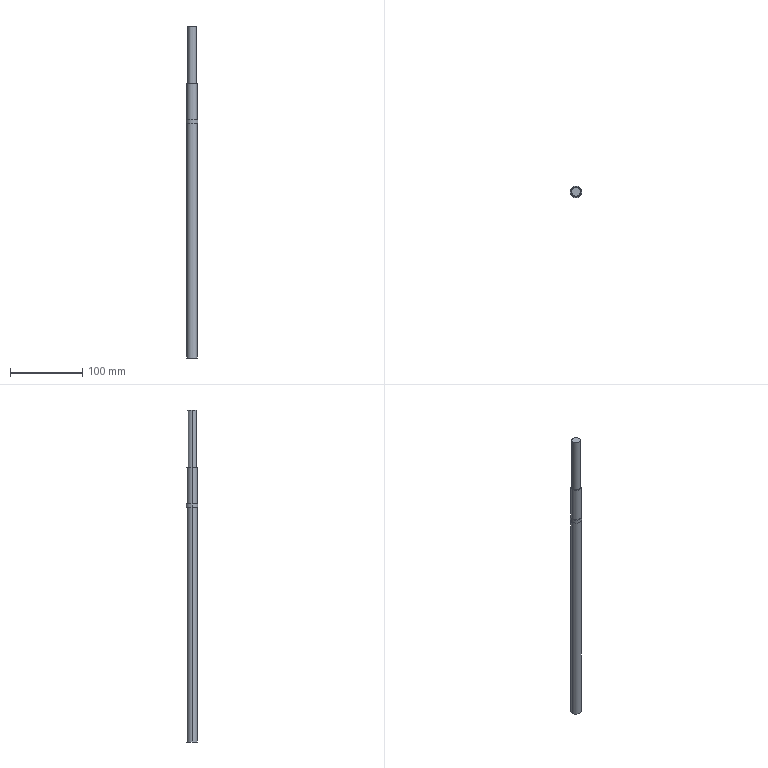Part | SolidWorks | features MirrorStock 1 | 1 solid | 13 faces | box 16 x 16 x 460 mm | volume 67780 mm3 | cylinder 8 | plane 5 | commonest cylinder face diameters 14 x4 12 x2 16 x2
STEP:
#1=CARTESIAN_POINT('',(-7.,0.,-460.));
#2=VERTEX_POINT('',#1);
#3=CARTESIAN_POINT('',(7.,0.,-460.));
#4=VERTEX_POINT('',#3);
#5=CARTESIAN_POINT('',(0.,0.,-460.));
#6=DIRECTION('',(0.,0.,1.));
#7=DIRECTION('',(1.,0.,0.));
#8=AXIS2_PLACEMENT_3D('',#5,#6,#7);
#9=CIRCLE('',#8,7.);
#10=EDGE_CURVE('',#2,#4,#9,.T.);
#11=ORIENTED_EDGE('',*,*,#10,.T.);
#12=CARTESIAN_POINT('',(7.,0.,-135.));
#13=VERTEX_POINT('',#12);
#14=CARTESIAN_POINT('',(7.,0.,-460.));
#15=DIRECTION('',(0.,0.,1.));
#16=VECTOR('',#15,1000.);
#17=LINE('',#14,#16);
#18=EDGE_CURVE('',#4,#13,#17,.T.);
#19=ORIENTED_EDGE('',*,*,#18,.T.);
#20=CARTESIAN_POINT('',(-7.,0.,-135.));
#21=VERTEX_POINT('',#20);
#22=CARTESIAN_POINT('',(0.,0.,-135.));
#23=DIRECTION('',(0.,0.,1.));
#24=DIRECTION('',(1.,0.,0.));
#25=AXIS2_PLACEMENT_3D('',#22,#23,#24);
#26=CIRCLE('',#25,7.);
#27=EDGE_CURVE('',#21,#13,#26,.T.);
#28=ORIENTED_EDGE('',*,*,#27,.F.);
#29=CARTESIAN_POINT('',(-7.,0.,-460.));
#30=DIRECTION('',(0.,0.,1.));
#31=VECTOR('',#30,1000.);
#32=LINE('',#29,#31);
#33=EDGE_CURVE('',#2,#21,#32,.T.);
#34=ORIENTED_EDGE('',*,*,#33,.F.);
#35=EDGE_LOOP('',(#11,#19,#28,#34));
#36=FACE_OUTER_BOUND('',#35,.T.);
#37=CARTESIAN_POINT('',(0.,0.,-460.));
#38=DIRECTION('',(0.,0.,1.));
#39=DIRECTION('',(-1.,0.,0.));
#40=AXIS2_PLACEMENT_3D('',#37,#38,#39);
#41=CYLINDRICAL_SURFACE('',#40,7.);
#42=ADVANCED_FACE('',(#36),#41,.T.);
#43=CARTESIAN_POINT('',(-8.,0.,-135.));
#44=VERTEX_POINT('',#43);
#45=CARTESIAN_POINT('',(8.,0.,-135.));
#46=VERTEX_POINT('',#45);
#47=CARTESIAN_POINT('',(0.,0.,-135.));
#48=DIRECTION('',(0.,0.,1.));
#49=DIRECTION('',(1.,0.,0.));
#50=AXIS2_PLACEMENT_3D('',#47,#48,#49);
#51=CIRCLE('',#50,8.);
#52=EDGE_CURVE('',#44,#46,#51,.T.);
#53=ORIENTED_EDGE('',*,*,#52,.T.);
#54=CARTESIAN_POINT('',(8.,0.,-130.));
#55=VERTEX_POINT('',#54);
#56=CARTESIAN_POINT('',(8.,0.,-135.));
#57=DIRECTION('',(0.,0.,1.));
#58=VECTOR('',#57,1000.);
#59=LINE('',#56,#58);
#60=EDGE_CURVE('',#46,#55,#59,.T.);
#61=ORIENTED_EDGE('',*,*,#60,.T.);
#62=CARTESIAN_POINT('',(-8.,0.,-130.));
#63=VERTEX_POINT('',#62);
#64=CARTESIAN_POINT('',(0.,0.,-130.));
#65=DIRECTION('',(0.,0.,1.));
#66=DIRECTION('',(1.,0.,0.));
#67=AXIS2_PLACEMENT_3D('',#64,#65,#66);
#68=CIRCLE('',#67,8.);
#69=EDGE_CURVE('',#63,#55,#68,.T.);
#70=ORIENTED_EDGE('',*,*,#69,.F.);
#71=CARTESIAN_POINT('',(-8.,0.,-135.));
#72=DIRECTION('',(0.,0.,1.));
#73=VECTOR('',#72,1000.);
#74=LINE('',#71,#73);
#75=EDGE_CURVE('',#44,#63,#74,.T.);
#76=ORIENTED_EDGE('',*,*,#75,.F.);
#77=EDGE_LOOP('',(#53,#61,#70,#76));
#78=FACE_OUTER_BOUND('',#77,.T.);
#79=CARTESIAN_POINT('',(0.,0.,-135.));
#80=DIRECTION('',(0.,0.,1.));
#81=DIRECTION('',(-1.,0.,0.));
#82=AXIS2_PLACEMENT_3D('',#79,#80,#81);
#83=CYLINDRICAL_SURFACE('',#82,8.);
#84=ADVANCED_FACE('',(#78),#83,.T.);
#85=CARTESIAN_POINT('',(-6.,0.,-80.));
#86=VERTEX_POINT('',#85);
#87=CARTESIAN_POINT('',(6.,0.,-80.));
#88=VERTEX_POINT('',#87);
#89=CARTESIAN_POINT('',(0.,0.,-80.));
#90=DIRECTION('',(0.,0.,1.));
#91=DIRECTION('',(1.,0.,0.));
#92=AXIS2_PLACEMENT_3D('',#89,#90,#91);
#93=CIRCLE('',#92,6.);
#94=EDGE_CURVE('',#86,#88,#93,.T.);
#95=ORIENTED_EDGE('',*,*,#94,.T.);
#96=CARTESIAN_POINT('',(6.,0.,0.));
#97=VERTEX_POINT('',#96);
#98=CARTESIAN_POINT('',(6.,0.,-80.));
#99=DIRECTION('',(0.,0.,1.));
#100=VECTOR('',#99,1000.);
#101=LINE('',#98,#100);
#102=EDGE_CURVE('',#88,#97,#101,.T.);
#103=ORIENTED_EDGE('',*,*,#102,.T.);
#104=CARTESIAN_POINT('',(-6.,0.,0.));
#105=VERTEX_POINT('',#104);
#106=CARTESIAN_POINT('',(0.,0.,0.));
#107=DIRECTION('',(0.,0.,1.));
#108=DIRECTION('',(1.,0.,0.));
#109=AXIS2_PLACEMENT_3D('',#106,#107,#108);
#110=CIRCLE('',#109,6.);
#111=EDGE_CURVE('',#105,#97,#110,.T.);
#112=ORIENTED_EDGE('',*,*,#111,.F.);
#113=CARTESIAN_POINT('',(-6.,0.,-80.));
#114=DIRECTION('',(0.,0.,1.));
#115=VECTOR('',#114,1000.);
#116=LINE('',#113,#115);
#117=EDGE_CURVE('',#86,#105,#116,.T.);
#118=ORIENTED_EDGE('',*,*,#117,.F.);
#119=EDGE_LOOP('',(#95,#103,#112,#118));
#120=FACE_OUTER_BOUND('',#119,.T.);
#121=CARTESIAN_POINT('',(0.,0.,-80.));
#122=DIRECTION('',(0.,0.,1.));
#123=DIRECTION('',(-1.,0.,0.));
#124=AXIS2_PLACEMENT_3D('',#121,#122,#123);
#125=CYLINDRICAL_SURFACE('',#124,6.);
#126=ADVANCED_FACE('',(#120),#125,.T.);
#127=CARTESIAN_POINT('',(-7.,0.,-130.));
#128=VERTEX_POINT('',#127);
#129=CARTESIAN_POINT('',(7.,0.,-130.));
#130=VERTEX_POINT('',#129);
#131=CARTESIAN_POINT('',(0.,0.,-130.));
#132=DIRECTION('',(0.,0.,1.));
#133=DIRECTION('',(1.,0.,0.));
#134=AXIS2_PLACEMENT_3D('',#131,#132,#133);
#135=CIRCLE('',#134,7.);
#136=EDGE_CURVE('',#128,#130,#135,.T.);
#137=ORIENTED_EDGE('',*,*,#136,.T.);
#138=CARTESIAN_POINT('',(7.,0.,-80.));
#139=VERTEX_POINT('',#138);
#140=CARTESIAN_POINT('',(7.,0.,-460.));
#141=DIRECTION('',(0.,0.,1.));
#142=VECTOR('',#141,1000.);
#143=LINE('',#140,#142);
#144=EDGE_CURVE('',#130,#139,#143,.T.);
#145=ORIENTED_EDGE('',*,*,#144,.T.);
#146=CARTESIAN_POINT('',(-7.,0.,-80.));
#147=VERTEX_POINT('',#146);
#148=CARTESIAN_POINT('',(0.,0.,-80.));
#149=DIRECTION('',(0.,0.,1.));
#150=DIRECTION('',(1.,0.,0.));
#151=AXIS2_PLACEMENT_3D('',#148,#149,#150);
#152=CIRCLE('',#151,7.);
#153=EDGE_CURVE('',#147,#139,#152,.T.);
#154=ORIENTED_EDGE('',*,*,#153,.F.);
#155=CARTESIAN_POINT('',(-7.,0.,-460.));
#156=DIRECTION('',(0.,0.,1.));
#157=VECTOR('',#156,1000.);
#158=LINE('',#155,#157);
#159=EDGE_CURVE('',#128,#147,#158,.T.);
#160=ORIENTED_EDGE('',*,*,#159,.F.);
#161=EDGE_LOOP('',(#137,#145,#154,#160));
#162=FACE_OUTER_BOUND('',#161,.T.);
#163=CARTESIAN_POINT('',(0.,0.,-460.));
#164=DIRECTION('',(0.,0.,1.));
#165=DIRECTION('',(-1.,0.,0.));
#166=AXIS2_PLACEMENT_3D('',#163,#164,#165);
#167=CYLINDRICAL_SURFACE('',#166,7.);
#168=ADVANCED_FACE('',(#162),#167,.T.);
#169=ORIENTED_EDGE('',*,*,#144,.F.);
#170=CARTESIAN_POINT('',(0.,0.,-130.));
#171=DIRECTION('',(0.,0.,1.));
#172=DIRECTION('',(1.,0.,0.));
#173=AXIS2_PLACEMENT_3D('',#170,#171,#172);
#174=CIRCLE('',#173,7.);
#175=EDGE_CURVE('',#130,#128,#174,.T.);
#176=ORIENTED_EDGE('',*,*,#175,.T.);
#177=ORIENTED_EDGE('',*,*,#159,.T.);
#178=CARTESIAN_POINT('',(0.,0.,-80.));
#179=DIRECTION('',(0.,0.,1.));
#180=DIRECTION('',(1.,0.,0.));
#181=AXIS2_PLACEMENT_3D('',#178,#179,#180);
#182=CIRCLE('',#181,7.);
#183=EDGE_CURVE('',#139,#147,#182,.T.);
#184=ORIENTED_EDGE('',*,*,#183,.F.);
#185=EDGE_LOOP('',(#169,#176,#177,#184));
#186=FACE_OUTER_BOUND('',#185,.T.);
#187=CARTESIAN_POINT('',(0.,0.,-460.));
#188=DIRECTION('',(0.,0.,1.));
#189=DIRECTION('',(-1.,0.,0.));
#190=AXIS2_PLACEMENT_3D('',#187,#188,#189);
#191=CYLINDRICAL_SURFACE('',#190,7.);
#192=ADVANCED_FACE('',(#186),#191,.T.);
#193=ORIENTED_EDGE('',*,*,#102,.F.);
#194=CARTESIAN_POINT('',(0.,0.,-80.));
#195=DIRECTION('',(0.,0.,1.));
#196=DIRECTION('',(1.,0.,0.));
#197=AXIS2_PLACEMENT_3D('',#194,#195,#196);
#198=CIRCLE('',#197,6.);
#199=EDGE_CURVE('',#88,#86,#198,.T.);
#200=ORIENTED_EDGE('',*,*,#199,.T.);
#201=ORIENTED_EDGE('',*,*,#117,.T.);
#202=CARTESIAN_POINT('',(0.,0.,0.));
#203=DIRECTION('',(0.,0.,1.));
#204=DIRECTION('',(1.,0.,0.));
#205=AXIS2_PLACEMENT_3D('',#202,#203,#204);
#206=CIRCLE('',#205,6.);
#207=EDGE_CURVE('',#97,#105,#206,.T.);
#208=ORIENTED_EDGE('',*,*,#207,.F.);
#209=EDGE_LOOP('',(#193,#200,#201,#208));
#210=FACE_OUTER_BOUND('',#209,.T.);
#211=CARTESIAN_POINT('',(0.,0.,-80.));
#212=DIRECTION('',(0.,0.,1.));
#213=DIRECTION('',(-1.,0.,0.));
#214=AXIS2_PLACEMENT_3D('',#211,#212,#213);
#215=CYLINDRICAL_SURFACE('',#214,6.);
#216=ADVANCED_FACE('',(#210),#215,.T.);
#217=ORIENTED_EDGE('',*,*,#111,.T.);
#218=ORIENTED_EDGE('',*,*,#207,.T.);
#219=EDGE_LOOP('',(#217,#218));
#220=FACE_OUTER_BOUND('',#219,.T.);
#221=CARTESIAN_POINT('',(0.,0.,0.));
#222=DIRECTION('',(0.,0.,-1.));
#223=DIRECTION('',(1.,0.,0.));
#224=AXIS2_PLACEMENT_3D('',#221,#222,#223);
#225=PLANE('',#224);
#226=ADVANCED_FACE('',(#220),#225,.F.);
#227=ORIENTED_EDGE('',*,*,#94,.F.);
#228=ORIENTED_EDGE('',*,*,#199,.F.);
#229=EDGE_LOOP('',(#227,#228));
#230=FACE_BOUND('',#229,.T.);
#231=ORIENTED_EDGE('',*,*,#153,.T.);
#232=ORIENTED_EDGE('',*,*,#183,.T.);
#233=EDGE_LOOP('',(#231,#232));
#234=FACE_OUTER_BOUND('',#233,.T.);
#235=CARTESIAN_POINT('',(0.,0.,-80.));
#236=DIRECTION('',(0.,0.,-1.));
#237=DIRECTION('',(1.,0.,0.));
#238=AXIS2_PLACEMENT_3D('',#235,#236,#237);
#239=PLANE('',#238);
#240=ADVANCED_FACE('',(#230,#234),#239,.F.);
#241=ORIENTED_EDGE('',*,*,#60,.F.);
#242=CARTESIAN_POINT('',(0.,0.,-135.));
#243=DIRECTION('',(0.,0.,1.));
#244=DIRECTION('',(1.,0.,0.));
#245=AXIS2_PLACEMENT_3D('',#242,#243,#244);
#246=CIRCLE('',#245,8.);
#247=EDGE_CURVE('',#46,#44,#246,.T.);
#248=ORIENTED_EDGE('',*,*,#247,.T.);
#249=ORIENTED_EDGE('',*,*,#75,.T.);
#250=CARTESIAN_POINT('',(0.,0.,-130.));
#251=DIRECTION('',(0.,0.,1.));
#252=DIRECTION('',(1.,0.,0.));
#253=AXIS2_PLACEMENT_3D('',#250,#251,#252);
#254=CIRCLE('',#253,8.);
#255=EDGE_CURVE('',#55,#63,#254,.T.);
#256=ORIENTED_EDGE('',*,*,#255,.F.);
#257=EDGE_LOOP('',(#241,#248,#249,#256));
#258=FACE_OUTER_BOUND('',#257,.T.);
#259=CARTESIAN_POINT('',(0.,0.,-135.));
#260=DIRECTION('',(0.,0.,1.));
#261=DIRECTION('',(-1.,0.,0.));
#262=AXIS2_PLACEMENT_3D('',#259,#260,#261);
#263=CYLINDRICAL_SURFACE('',#262,8.);
#264=ADVANCED_FACE('',(#258),#263,.T.);
#265=ORIENTED_EDGE('',*,*,#27,.T.);
#266=CARTESIAN_POINT('',(0.,0.,-135.));
#267=DIRECTION('',(0.,0.,1.));
#268=DIRECTION('',(1.,0.,0.));
#269=AXIS2_PLACEMENT_3D('',#266,#267,#268);
#270=CIRCLE('',#269,7.);
#271=EDGE_CURVE('',#13,#21,#270,.T.);
#272=ORIENTED_EDGE('',*,*,#271,.T.);
#273=EDGE_LOOP('',(#265,#272));
#274=FACE_BOUND('',#273,.T.);
#275=ORIENTED_EDGE('',*,*,#52,.F.);
#276=ORIENTED_EDGE('',*,*,#247,.F.);
#277=EDGE_LOOP('',(#275,#276));
#278=FACE_OUTER_BOUND('',#277,.T.);
#279=CARTESIAN_POINT('',(0.,0.,-135.));
#280=DIRECTION('',(0.,0.,-1.));
#281=DIRECTION('',(1.,0.,0.));
#282=AXIS2_PLACEMENT_3D('',#279,#280,#281);
#283=PLANE('',#282);
#284=ADVANCED_FACE('',(#274,#278),#283,.T.);
#285=ORIENTED_EDGE('',*,*,#136,.F.);
#286=ORIENTED_EDGE('',*,*,#175,.F.);
#287=EDGE_LOOP('',(#285,#286));
#288=FACE_BOUND('',#287,.T.);
#289=ORIENTED_EDGE('',*,*,#69,.T.);
#290=ORIENTED_EDGE('',*,*,#255,.T.);
#291=EDGE_LOOP('',(#289,#290));
#292=FACE_OUTER_BOUND('',#291,.T.);
#293=CARTESIAN_POINT('',(0.,0.,-130.));
#294=DIRECTION('',(0.,0.,-1.));
#295=DIRECTION('',(1.,0.,0.));
#296=AXIS2_PLACEMENT_3D('',#293,#294,#295);
#297=PLANE('',#296);
#298=ADVANCED_FACE('',(#288,#292),#297,.F.);
#299=ORIENTED_EDGE('',*,*,#10,.F.);
#300=CARTESIAN_POINT('',(0.,0.,-460.));
#301=DIRECTION('',(0.,0.,1.));
#302=DIRECTION('',(1.,0.,0.));
#303=AXIS2_PLACEMENT_3D('',#300,#301,#302);
#304=CIRCLE('',#303,7.);
#305=EDGE_CURVE('',#4,#2,#304,.T.);
#306=ORIENTED_EDGE('',*,*,#305,.F.);
#307=EDGE_LOOP('',(#299,#306));
#308=FACE_OUTER_BOUND('',#307,.T.);
#309=CARTESIAN_POINT('',(0.,0.,-460.));
#310=DIRECTION('',(0.,0.,-1.));
#311=DIRECTION('',(1.,0.,0.));
#312=AXIS2_PLACEMENT_3D('',#309,#310,#311);
#313=PLANE('',#312);
#314=ADVANCED_FACE('',(#308),#313,.T.);
#315=ORIENTED_EDGE('',*,*,#18,.F.);
#316=ORIENTED_EDGE('',*,*,#305,.T.);
#317=ORIENTED_EDGE('',*,*,#33,.T.);
#318=ORIENTED_EDGE('',*,*,#271,.F.);
#319=EDGE_LOOP('',(#315,#316,#317,#318));
#320=FACE_OUTER_BOUND('',#319,.T.);
#321=CARTESIAN_POINT('',(0.,0.,-460.));
#322=DIRECTION('',(0.,0.,1.));
#323=DIRECTION('',(-1.,0.,0.));
#324=AXIS2_PLACEMENT_3D('',#321,#322,#323);
#325=CYLINDRICAL_SURFACE('',#324,7.);
#326=ADVANCED_FACE('',(#320),#325,.T.);
#327=CLOSED_SHELL('',(#42,#84,#126,#168,#192,#216,#226,#240,#264,#284,#298,#314,#326));
#328=MANIFOLD_SOLID_BREP('',#327);
#329=CARTESIAN_POINT('',(0.,0.,0.));
#330=DIRECTION('',(0.,0.,1.));
#331=DIRECTION('',(1.,0.,0.));
#332=AXIS2_PLACEMENT_3D('',#329,#330,#331);
#333=(LENGTH_UNIT()NAMED_UNIT(*)SI_UNIT(.MILLI.,.METRE.));
#334=UNCERTAINTY_MEASURE_WITH_UNIT(LENGTH_MEASURE(0.00001),#333,'','');
#335=(NAMED_UNIT(*)PLANE_ANGLE_UNIT()SI_UNIT($,.RADIAN.));
#336=(NAMED_UNIT(*)SI_UNIT($,.STERADIAN.)SOLID_ANGLE_UNIT());
#337=(GEOMETRIC_REPRESENTATION_CONTEXT(3)GLOBAL_UNCERTAINTY_ASSIGNED_CONTEXT((#334))GLOBAL_UNIT_ASSIGNED_CONTEXT((#333,#335,#336))REPRESENTATION_CONTEXT('',''));
#338=ADVANCED_BREP_SHAPE_REPRESENTATION('',(#328,#332),#337);